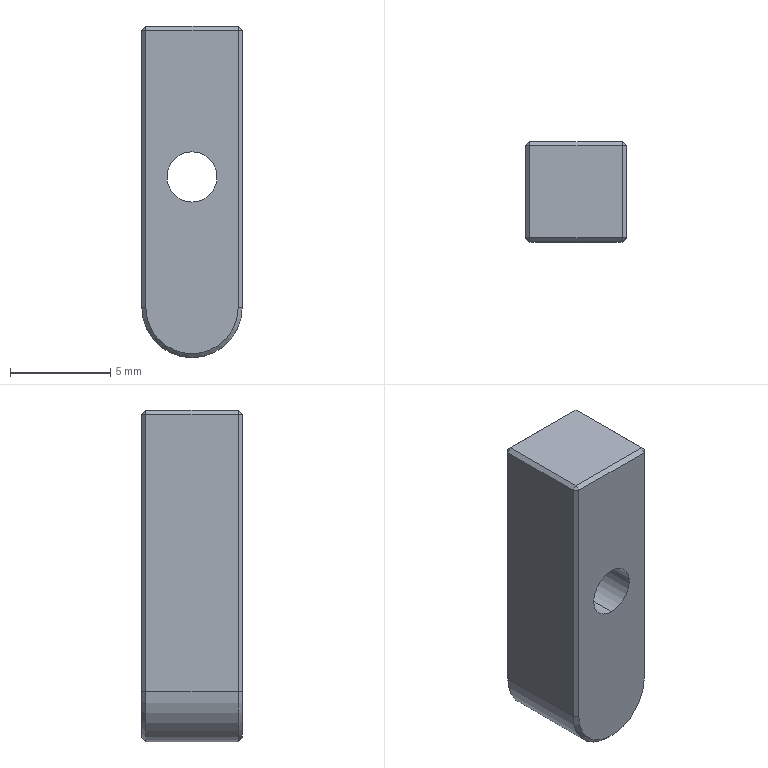Part | STEP file | 22010150--1-SOLI00_1_1_1 | 1 solid | 25 faces | box 5 x 5 x 16.5 mm | volume 372.42 mm3 | plane 17 | cone 5 | cylinder 3 | commonest cylinder face diameters 2.5 x2 5 x1
STEP:
#1=CARTESIAN_POINT('',(0.,0.,0.));
#2=DIRECTION('',(0.,0.,1.));
#3=DIRECTION('',(1.,0.,0.));
#4=AXIS2_PLACEMENT_3D('',#1,#2,#3);
#5=CARTESIAN_POINT('',(0.,4.,23.75));
#6=VERTEX_POINT('',#5);
#7=CARTESIAN_POINT('',(0.,8.725,23.75));
#8=VERTEX_POINT('',#7);
#9=CARTESIAN_POINT('',(0.,9.,23.75));
#10=DIRECTION('',(0.,1.,0.));
#11=VECTOR('',#10,1.);
#12=LINE('',#9,#11);
#13=CARTESIAN_POINT('',(0.,9.,22.5));
#14=DIRECTION('',(0.,1.,0.));
#15=DIRECTION('',(0.,0.,1.));
#16=AXIS2_PLACEMENT_3D('',#13,#14,#15);
#17=CYLINDRICAL_SURFACE('',#16,1.25);
#18=CARTESIAN_POINT('',(6.283,0.));
#19=DIRECTION('',(0.,1.));
#20=VECTOR('',#19,1.);
#21=LINE('',#18,#20);
#22=(GEOMETRIC_REPRESENTATION_CONTEXT(2)PARAMETRIC_REPRESENTATION_CONTEXT()REPRESENTATION_CONTEXT('',''));
#23=DEFINITIONAL_REPRESENTATION('',(#21),#22);
#24=PCURVE('',#17,#23);
#25=CARTESIAN_POINT('',(0.,9.,22.5));
#26=DIRECTION('',(0.,1.,0.));
#27=DIRECTION('',(0.,0.,1.));
#28=AXIS2_PLACEMENT_3D('',#25,#26,#27);
#29=CYLINDRICAL_SURFACE('',#28,1.25);
#30=CARTESIAN_POINT('',(0.,0.));
#31=DIRECTION('',(0.,1.));
#32=VECTOR('',#31,1.);
#33=LINE('',#30,#32);
#34=(GEOMETRIC_REPRESENTATION_CONTEXT(2)PARAMETRIC_REPRESENTATION_CONTEXT()REPRESENTATION_CONTEXT('',''));
#35=DEFINITIONAL_REPRESENTATION('',(#33),#34);
#36=PCURVE('',#29,#35);
#37=SURFACE_CURVE('',#12,(#24,#36),.PCURVE_S1.);
#38=EDGE_CURVE('',#6,#8,#37,.T.);
#39=ORIENTED_EDGE('',*,*,#38,.T.);
#40=CARTESIAN_POINT('',(0.,8.725,21.25));
#41=VERTEX_POINT('',#40);
#42=CARTESIAN_POINT('',(0.,8.725,22.5));
#43=DIRECTION('',(0.,-1.,0.));
#44=DIRECTION('',(0.,0.,1.));
#45=AXIS2_PLACEMENT_3D('',#42,#43,#44);
#46=CIRCLE('',#45,1.25);
#47=CARTESIAN_POINT('',(6.283,-0.275));
#48=DIRECTION('',(-1.,0.));
#49=VECTOR('',#48,1.);
#50=LINE('',#47,#49);
#51=(GEOMETRIC_REPRESENTATION_CONTEXT(2)PARAMETRIC_REPRESENTATION_CONTEXT()REPRESENTATION_CONTEXT('',''));
#52=DEFINITIONAL_REPRESENTATION('',(#50),#51);
#53=PCURVE('',#17,#52);
#54=CARTESIAN_POINT('',(0.,9.,22.5));
#55=DIRECTION('',(0.,1.,0.));
#56=DIRECTION('',(0.,0.,1.));
#57=AXIS2_PLACEMENT_3D('',#54,#55,#56);
#58=CONICAL_SURFACE('',#57,1.525,0.7854);
#59=CARTESIAN_POINT('',(6.283,-0.275));
#60=DIRECTION('',(-1.,0.));
#61=VECTOR('',#60,1.);
#62=LINE('',#59,#61);
#63=(GEOMETRIC_REPRESENTATION_CONTEXT(2)PARAMETRIC_REPRESENTATION_CONTEXT()REPRESENTATION_CONTEXT('',''));
#64=DEFINITIONAL_REPRESENTATION('',(#62),#63);
#65=PCURVE('',#58,#64);
#66=SURFACE_CURVE('',#46,(#53,#65),.PCURVE_S1.);
#67=EDGE_CURVE('',#8,#41,#66,.T.);
#68=ORIENTED_EDGE('',*,*,#67,.T.);
#69=CARTESIAN_POINT('',(0.,4.,21.25));
#70=VERTEX_POINT('',#69);
#71=CARTESIAN_POINT('',(0.,9.,21.25));
#72=DIRECTION('',(0.,1.,0.));
#73=VECTOR('',#72,1.);
#74=LINE('',#71,#73);
#75=CARTESIAN_POINT('',(3.142,0.));
#76=DIRECTION('',(0.,1.));
#77=VECTOR('',#76,1.);
#78=LINE('',#75,#77);
#79=(GEOMETRIC_REPRESENTATION_CONTEXT(2)PARAMETRIC_REPRESENTATION_CONTEXT()REPRESENTATION_CONTEXT('',''));
#80=DEFINITIONAL_REPRESENTATION('',(#78),#79);
#81=PCURVE('',#17,#80);
#82=CARTESIAN_POINT('',(3.142,0.));
#83=DIRECTION('',(0.,1.));
#84=VECTOR('',#83,1.);
#85=LINE('',#82,#84);
#86=(GEOMETRIC_REPRESENTATION_CONTEXT(2)PARAMETRIC_REPRESENTATION_CONTEXT()REPRESENTATION_CONTEXT('',''));
#87=DEFINITIONAL_REPRESENTATION('',(#85),#86);
#88=PCURVE('',#29,#87);
#89=SURFACE_CURVE('',#74,(#81,#88),.PCURVE_S1.);
#90=EDGE_CURVE('',#70,#41,#89,.T.);
#91=ORIENTED_EDGE('',*,*,#90,.F.);
#92=CARTESIAN_POINT('',(0.,4.,22.5));
#93=DIRECTION('',(0.,1.,0.));
#94=DIRECTION('',(0.,0.,1.));
#95=AXIS2_PLACEMENT_3D('',#92,#93,#94);
#96=CIRCLE('',#95,1.25);
#97=CARTESIAN_POINT('',(0.,-5.));
#98=DIRECTION('',(1.,0.));
#99=VECTOR('',#98,1.);
#100=LINE('',#97,#99);
#101=(GEOMETRIC_REPRESENTATION_CONTEXT(2)PARAMETRIC_REPRESENTATION_CONTEXT()REPRESENTATION_CONTEXT('',''));
#102=DEFINITIONAL_REPRESENTATION('',(#100),#101);
#103=PCURVE('',#17,#102);
#104=CARTESIAN_POINT('',(0.,4.,16.));
#105=DIRECTION('',(0.,-1.,0.));
#106=DIRECTION('',(0.,0.,-1.));
#107=AXIS2_PLACEMENT_3D('',#104,#105,#106);
#108=PLANE('',#107);
#109=CARTESIAN_POINT('',(-7.75,0.));
#110=CARTESIAN_POINT('',(-7.75,2.165));
#111=CARTESIAN_POINT('',(-5.875,1.083));
#112=CARTESIAN_POINT('',(-4.,0.));
#113=CARTESIAN_POINT('',(-5.875,-1.083));
#114=CARTESIAN_POINT('',(-7.75,-2.165));
#115=CARTESIAN_POINT('',(-7.75,0.));
#116=(BOUNDED_CURVE()B_SPLINE_CURVE(2,(#109,#110,#111,#112,#113,#114,#115),.UNSPECIFIED.,.T.,.F.)B_SPLINE_CURVE_WITH_KNOTS((1,2,2,2,2,1),(-2.094,0.,2.094,4.189,6.283,8.378),.UNSPECIFIED.)CURVE()GEOMETRIC_REPRESENTATION_ITEM()RATIONAL_B_SPLINE_CURVE((1.,0.5,1.,0.5,1.,0.5,1.))REPRESENTATION_ITEM(''));
#117=(GEOMETRIC_REPRESENTATION_CONTEXT(2)PARAMETRIC_REPRESENTATION_CONTEXT()REPRESENTATION_CONTEXT('',''));
#118=DEFINITIONAL_REPRESENTATION('',(#116),#117);
#119=PCURVE('',#108,#118);
#120=SURFACE_CURVE('',#96,(#103,#119),.PCURVE_S1.);
#121=EDGE_CURVE('',#70,#6,#120,.T.);
#122=ORIENTED_EDGE('',*,*,#121,.T.);
#123=EDGE_LOOP('',(#39,#68,#91,#122));
#124=FACE_BOUND('',#123,.F.);
#125=ADVANCED_FACE('',(#124),#17,.F.);
#126=CARTESIAN_POINT('',(0.,9.,24.025));
#127=VERTEX_POINT('',#126);
#128=CARTESIAN_POINT('',(0.,9.,24.025));
#129=DIRECTION('',(0.,0.7071,0.7071));
#130=VECTOR('',#129,1.);
#131=LINE('',#128,#130);
#132=CARTESIAN_POINT('',(6.283,0.));
#133=DIRECTION('',(0.,1.));
#134=VECTOR('',#133,1.);
#135=LINE('',#132,#134);
#136=(GEOMETRIC_REPRESENTATION_CONTEXT(2)PARAMETRIC_REPRESENTATION_CONTEXT()REPRESENTATION_CONTEXT('',''));
#137=DEFINITIONAL_REPRESENTATION('',(#135),#136);
#138=PCURVE('',#58,#137);
#139=CARTESIAN_POINT('',(0.,9.,22.5));
#140=DIRECTION('',(0.,1.,0.));
#141=DIRECTION('',(0.,0.,1.));
#142=AXIS2_PLACEMENT_3D('',#139,#140,#141);
#143=CONICAL_SURFACE('',#142,1.525,0.7854);
#144=CARTESIAN_POINT('',(0.,0.));
#145=DIRECTION('',(0.,1.));
#146=VECTOR('',#145,1.);
#147=LINE('',#144,#146);
#148=(GEOMETRIC_REPRESENTATION_CONTEXT(2)PARAMETRIC_REPRESENTATION_CONTEXT()REPRESENTATION_CONTEXT('',''));
#149=DEFINITIONAL_REPRESENTATION('',(#147),#148);
#150=PCURVE('',#143,#149);
#151=SURFACE_CURVE('',#131,(#138,#150),.PCURVE_S1.);
#152=EDGE_CURVE('',#8,#127,#151,.T.);
#153=ORIENTED_EDGE('',*,*,#152,.T.);
#154=CARTESIAN_POINT('',(0.,9.,20.975));
#155=VERTEX_POINT('',#154);
#156=CARTESIAN_POINT('',(0.,9.,22.5));
#157=DIRECTION('',(0.,-1.,0.));
#158=DIRECTION('',(0.,0.,1.));
#159=AXIS2_PLACEMENT_3D('',#156,#157,#158);
#160=CIRCLE('',#159,1.525);
#161=CARTESIAN_POINT('',(6.283,0.));
#162=DIRECTION('',(-1.,0.));
#163=VECTOR('',#162,1.);
#164=LINE('',#161,#163);
#165=(GEOMETRIC_REPRESENTATION_CONTEXT(2)PARAMETRIC_REPRESENTATION_CONTEXT()REPRESENTATION_CONTEXT('',''));
#166=DEFINITIONAL_REPRESENTATION('',(#164),#165);
#167=PCURVE('',#58,#166);
#168=CARTESIAN_POINT('',(0.,9.,16.));
#169=DIRECTION('',(0.,-1.,0.));
#170=DIRECTION('',(0.,0.,-1.));
#171=AXIS2_PLACEMENT_3D('',#168,#169,#170);
#172=PLANE('',#171);
#173=CARTESIAN_POINT('',(-6.5,0.));
#174=DIRECTION('',(-1.,0.));
#175=AXIS2_PLACEMENT_2D('',#173,#174);
#176=CIRCLE('',#175,1.525);
#177=(GEOMETRIC_REPRESENTATION_CONTEXT(2)PARAMETRIC_REPRESENTATION_CONTEXT()REPRESENTATION_CONTEXT('',''));
#178=DEFINITIONAL_REPRESENTATION('',(#176),#177);
#179=PCURVE('',#172,#178);
#180=SURFACE_CURVE('',#160,(#167,#179),.PCURVE_S1.);
#181=EDGE_CURVE('',#127,#155,#180,.T.);
#182=ORIENTED_EDGE('',*,*,#181,.T.);
#183=CARTESIAN_POINT('',(0.,9.,20.975));
#184=DIRECTION('',(0.,0.7071,-0.7071));
#185=VECTOR('',#184,1.);
#186=LINE('',#183,#185);
#187=CARTESIAN_POINT('',(3.142,0.));
#188=DIRECTION('',(0.,1.));
#189=VECTOR('',#188,1.);
#190=LINE('',#187,#189);
#191=(GEOMETRIC_REPRESENTATION_CONTEXT(2)PARAMETRIC_REPRESENTATION_CONTEXT()REPRESENTATION_CONTEXT('',''));
#192=DEFINITIONAL_REPRESENTATION('',(#190),#191);
#193=PCURVE('',#58,#192);
#194=CARTESIAN_POINT('',(3.142,0.));
#195=DIRECTION('',(0.,1.));
#196=VECTOR('',#195,1.);
#197=LINE('',#194,#196);
#198=(GEOMETRIC_REPRESENTATION_CONTEXT(2)PARAMETRIC_REPRESENTATION_CONTEXT()REPRESENTATION_CONTEXT('',''));
#199=DEFINITIONAL_REPRESENTATION('',(#197),#198);
#200=PCURVE('',#143,#199);
#201=SURFACE_CURVE('',#186,(#193,#200),.PCURVE_S1.);
#202=EDGE_CURVE('',#41,#155,#201,.T.);
#203=ORIENTED_EDGE('',*,*,#202,.F.);
#204=ORIENTED_EDGE('',*,*,#67,.F.);
#205=EDGE_LOOP('',(#153,#182,#203,#204));
#206=FACE_BOUND('',#205,.F.);
#207=ADVANCED_FACE('',(#206),#58,.F.);
#208=CARTESIAN_POINT('',(-2.3,9.,16.));
#209=VERTEX_POINT('',#208);
#210=CARTESIAN_POINT('',(0.,9.,13.7));
#211=VERTEX_POINT('',#210);
#212=CARTESIAN_POINT('',(0.,9.,16.));
#213=DIRECTION('',(0.,-1.,0.));
#214=DIRECTION('',(0.,0.,-1.));
#215=AXIS2_PLACEMENT_3D('',#212,#213,#214);
#216=CIRCLE('',#215,2.3);
#217=CARTESIAN_POINT('',(0.,8.8,16.));
#218=DIRECTION('',(0.,-1.,0.));
#219=DIRECTION('',(0.,0.,-1.));
#220=AXIS2_PLACEMENT_3D('',#217,#218,#219);
#221=CONICAL_SURFACE('',#220,2.5,0.7854);
#222=CARTESIAN_POINT('',(0.,-0.2));
#223=DIRECTION('',(1.,0.));
#224=VECTOR('',#223,1.);
#225=LINE('',#222,#224);
#226=(GEOMETRIC_REPRESENTATION_CONTEXT(2)PARAMETRIC_REPRESENTATION_CONTEXT()REPRESENTATION_CONTEXT('',''));
#227=DEFINITIONAL_REPRESENTATION('',(#225),#226);
#228=PCURVE('',#221,#227);
#229=CARTESIAN_POINT('',(0.,0.));
#230=DIRECTION('',(1.,0.));
#231=AXIS2_PLACEMENT_2D('',#229,#230);
#232=CIRCLE('',#231,2.3);
#233=(GEOMETRIC_REPRESENTATION_CONTEXT(2)PARAMETRIC_REPRESENTATION_CONTEXT()REPRESENTATION_CONTEXT('',''));
#234=DEFINITIONAL_REPRESENTATION('',(#232),#233);
#235=PCURVE('',#172,#234);
#236=SURFACE_CURVE('',#216,(#228,#235),.PCURVE_S1.);
#237=EDGE_CURVE('',#209,#211,#236,.T.);
#238=ORIENTED_EDGE('',*,*,#237,.T.);
#239=CARTESIAN_POINT('',(0.,8.8,13.5));
#240=VERTEX_POINT('',#239);
#241=CARTESIAN_POINT('',(0.,8.8,13.5));
#242=DIRECTION('',(0.,-0.7071,-0.7071));
#243=VECTOR('',#242,1.);
#244=LINE('',#241,#243);
#245=CARTESIAN_POINT('',(6.283,0.));
#246=DIRECTION('',(0.,1.));
#247=VECTOR('',#246,1.);
#248=LINE('',#245,#247);
#249=(GEOMETRIC_REPRESENTATION_CONTEXT(2)PARAMETRIC_REPRESENTATION_CONTEXT()REPRESENTATION_CONTEXT('',''));
#250=DEFINITIONAL_REPRESENTATION('',(#248),#249);
#251=PCURVE('',#221,#250);
#252=CARTESIAN_POINT('',(0.,8.8,16.));
#253=DIRECTION('',(0.,-1.,0.));
#254=DIRECTION('',(0.,0.,-1.));
#255=AXIS2_PLACEMENT_3D('',#252,#253,#254);
#256=CONICAL_SURFACE('',#255,2.5,0.7854);
#257=CARTESIAN_POINT('',(0.,0.));
#258=DIRECTION('',(0.,1.));
#259=VECTOR('',#258,1.);
#260=LINE('',#257,#259);
#261=(GEOMETRIC_REPRESENTATION_CONTEXT(2)PARAMETRIC_REPRESENTATION_CONTEXT()REPRESENTATION_CONTEXT('',''));
#262=DEFINITIONAL_REPRESENTATION('',(#260),#261);
#263=PCURVE('',#256,#262);
#264=SURFACE_CURVE('',#244,(#251,#263),.PCURVE_S1.);
#265=EDGE_CURVE('',#211,#240,#264,.T.);
#266=ORIENTED_EDGE('',*,*,#265,.T.);
#267=CARTESIAN_POINT('',(-2.5,8.8,16.));
#268=VERTEX_POINT('',#267);
#269=CARTESIAN_POINT('',(0.,8.8,16.));
#270=DIRECTION('',(0.,-1.,0.));
#271=DIRECTION('',(0.,0.,1.));
#272=AXIS2_PLACEMENT_3D('',#269,#270,#271);
#273=CIRCLE('',#272,2.5);
#274=CARTESIAN_POINT('',(3.142,0.));
#275=DIRECTION('',(1.,0.));
#276=VECTOR('',#275,1.);
#277=LINE('',#274,#276);
#278=(GEOMETRIC_REPRESENTATION_CONTEXT(2)PARAMETRIC_REPRESENTATION_CONTEXT()REPRESENTATION_CONTEXT('',''));
#279=DEFINITIONAL_REPRESENTATION('',(#277),#278);
#280=PCURVE('',#221,#279);
#281=CARTESIAN_POINT('',(0.,4.,16.));
#282=DIRECTION('',(0.,1.,0.));
#283=DIRECTION('',(0.,0.,1.));
#284=AXIS2_PLACEMENT_3D('',#281,#282,#283);
#285=CYLINDRICAL_SURFACE('',#284,2.5);
#286=CARTESIAN_POINT('',(6.283,4.8));
#287=DIRECTION('',(-1.,0.));
#288=VECTOR('',#287,1.);
#289=LINE('',#286,#288);
#290=(GEOMETRIC_REPRESENTATION_CONTEXT(2)PARAMETRIC_REPRESENTATION_CONTEXT()REPRESENTATION_CONTEXT('',''));
#291=DEFINITIONAL_REPRESENTATION('',(#289),#290);
#292=PCURVE('',#285,#291);
#293=SURFACE_CURVE('',#273,(#280,#292),.PCURVE_S1.);
#294=EDGE_CURVE('',#268,#240,#293,.T.);
#295=ORIENTED_EDGE('',*,*,#294,.F.);
#296=CARTESIAN_POINT('',(-498984.,-498972.7,16.));
#297=DIRECTION('',(0.7071,0.7071,0.));
#298=VECTOR('',#297,1.);
#299=LINE('',#296,#298);
#300=CARTESIAN_POINT('',(4.712,498981.5));
#301=DIRECTION('',(0.,-1.));
#302=VECTOR('',#301,1.);
#303=LINE('',#300,#302);
#304=(GEOMETRIC_REPRESENTATION_CONTEXT(2)PARAMETRIC_REPRESENTATION_CONTEXT()REPRESENTATION_CONTEXT('',''));
#305=DEFINITIONAL_REPRESENTATION('',(#303),#304);
#306=PCURVE('',#221,#305);
#307=CARTESIAN_POINT('',(-2.5,8.8,16.));
#308=DIRECTION('',(0.7071,-0.7071,0.));
#309=DIRECTION('',(0.7071,0.7071,0.));
#310=AXIS2_PLACEMENT_3D('',#307,#308,#309);
#311=PLANE('',#310);
#312=CARTESIAN_POINT('',(-705666.405,0.));
#313=DIRECTION('',(1.,0.));
#314=VECTOR('',#313,1.);
#315=LINE('',#312,#314);
#316=(GEOMETRIC_REPRESENTATION_CONTEXT(2)PARAMETRIC_REPRESENTATION_CONTEXT()REPRESENTATION_CONTEXT('',''));
#317=DEFINITIONAL_REPRESENTATION('',(#315),#316);
#318=PCURVE('',#311,#317);
#319=SURFACE_CURVE('',#299,(#306,#318),.PCURVE_S1.);
#320=EDGE_CURVE('',#268,#209,#319,.T.);
#321=ORIENTED_EDGE('',*,*,#320,.T.);
#322=EDGE_LOOP('',(#238,#266,#295,#321));
#323=FACE_BOUND('',#322,.T.);
#324=ADVANCED_FACE('',(#323),#221,.T.);
#325=CARTESIAN_POINT('',(0.,4.,22.5));
#326=DIRECTION('',(0.,1.,0.));
#327=DIRECTION('',(0.,0.,1.));
#328=AXIS2_PLACEMENT_3D('',#325,#326,#327);
#329=CIRCLE('',#328,1.25);
#330=CARTESIAN_POINT('',(-7.75,0.));
#331=CARTESIAN_POINT('',(-7.75,2.165));
#332=CARTESIAN_POINT('',(-5.875,1.083));
#333=CARTESIAN_POINT('',(-4.,0.));
#334=CARTESIAN_POINT('',(-5.875,-1.083));
#335=CARTESIAN_POINT('',(-7.75,-2.165));
#336=CARTESIAN_POINT('',(-7.75,0.));
#337=(BOUNDED_CURVE()B_SPLINE_CURVE(2,(#330,#331,#332,#333,#334,#335,#336),.UNSPECIFIED.,.T.,.F.)B_SPLINE_CURVE_WITH_KNOTS((1,2,2,2,2,1),(-2.094,0.,2.094,4.189,6.283,8.378),.UNSPECIFIED.)CURVE()GEOMETRIC_REPRESENTATION_ITEM()RATIONAL_B_SPLINE_CURVE((1.,0.5,1.,0.5,1.,0.5,1.))REPRESENTATION_ITEM(''));
#338=(GEOMETRIC_REPRESENTATION_CONTEXT(2)PARAMETRIC_REPRESENTATION_CONTEXT()REPRESENTATION_CONTEXT('',''));
#339=DEFINITIONAL_REPRESENTATION('',(#337),#338);
#340=PCURVE('',#108,#339);
#341=CARTESIAN_POINT('',(0.,-5.));
#342=DIRECTION('',(1.,0.));
#343=VECTOR('',#342,1.);
#344=LINE('',#341,#343);
#345=(GEOMETRIC_REPRESENTATION_CONTEXT(2)PARAMETRIC_REPRESENTATION_CONTEXT()REPRESENTATION_CONTEXT('',''));
#346=DEFINITIONAL_REPRESENTATION('',(#344),#345);
#347=PCURVE('',#29,#346);
#348=SURFACE_CURVE('',#329,(#340,#347),.PCURVE_S1.);
#349=EDGE_CURVE('',#6,#70,#348,.T.);
#350=ORIENTED_EDGE('',*,*,#349,.T.);
#351=ORIENTED_EDGE('',*,*,#121,.T.);
#352=EDGE_LOOP('',(#350,#351));
#353=FACE_BOUND('',#352,.T.);
#354=CARTESIAN_POINT('',(2.3,4.,16.));
#355=VERTEX_POINT('',#354);
#356=CARTESIAN_POINT('',(2.3,4.,29.8));
#357=VERTEX_POINT('',#356);
#358=CARTESIAN_POINT('',(2.3,4.,16.));
#359=DIRECTION('',(0.,0.,1.));
#360=VECTOR('',#359,1.);
#361=LINE('',#358,#360);
#362=CARTESIAN_POINT('',(0.,2.3));
#363=DIRECTION('',(-1.,0.));
#364=VECTOR('',#363,1.);
#365=LINE('',#362,#364);
#366=(GEOMETRIC_REPRESENTATION_CONTEXT(2)PARAMETRIC_REPRESENTATION_CONTEXT()REPRESENTATION_CONTEXT('',''));
#367=DEFINITIONAL_REPRESENTATION('',(#365),#366);
#368=PCURVE('',#108,#367);
#369=CARTESIAN_POINT('',(2.3,4.,16.));
#370=DIRECTION('',(0.7071,-0.7071,0.));
#371=DIRECTION('',(0.7071,0.7071,0.));
#372=AXIS2_PLACEMENT_3D('',#369,#370,#371);
#373=PLANE('',#372);
#374=CARTESIAN_POINT('',(0.,0.));
#375=DIRECTION('',(0.,1.));
#376=VECTOR('',#375,1.);
#377=LINE('',#374,#376);
#378=(GEOMETRIC_REPRESENTATION_CONTEXT(2)PARAMETRIC_REPRESENTATION_CONTEXT()REPRESENTATION_CONTEXT('',''));
#379=DEFINITIONAL_REPRESENTATION('',(#377),#378);
#380=PCURVE('',#373,#379);
#381=SURFACE_CURVE('',#361,(#368,#380),.PCURVE_S1.);
#382=EDGE_CURVE('',#355,#357,#381,.T.);
#383=ORIENTED_EDGE('',*,*,#382,.T.);
#384=CARTESIAN_POINT('',(-2.3,4.,29.8));
#385=VERTEX_POINT('',#384);
#386=CARTESIAN_POINT('',(0.,4.,29.8));
#387=DIRECTION('',(-1.,0.,0.));
#388=VECTOR('',#387,1.);
#389=LINE('',#386,#388);
#390=CARTESIAN_POINT('',(-13.8,0.));
#391=DIRECTION('',(0.,-1.));
#392=VECTOR('',#391,1.);
#393=LINE('',#390,#392);
#394=(GEOMETRIC_REPRESENTATION_CONTEXT(2)PARAMETRIC_REPRESENTATION_CONTEXT()REPRESENTATION_CONTEXT('',''));
#395=DEFINITIONAL_REPRESENTATION('',(#393),#394);
#396=PCURVE('',#108,#395);
#397=CARTESIAN_POINT('',(0.,4.,29.8));
#398=DIRECTION('',(0.,-0.7071,0.7071));
#399=DIRECTION('',(0.,-0.7071,-0.7071));
#400=AXIS2_PLACEMENT_3D('',#397,#398,#399);
#401=PLANE('',#400);
#402=CARTESIAN_POINT('',(0.,0.));
#403=DIRECTION('',(0.,-1.));
#404=VECTOR('',#403,1.);
#405=LINE('',#402,#404);
#406=(GEOMETRIC_REPRESENTATION_CONTEXT(2)PARAMETRIC_REPRESENTATION_CONTEXT()REPRESENTATION_CONTEXT('',''));
#407=DEFINITIONAL_REPRESENTATION('',(#405),#406);
#408=PCURVE('',#401,#407);
#409=SURFACE_CURVE('',#389,(#396,#408),.PCURVE_S1.);
#410=EDGE_CURVE('',#357,#385,#409,.T.);
#411=ORIENTED_EDGE('',*,*,#410,.T.);
#412=CARTESIAN_POINT('',(-2.3,4.,16.));
#413=VERTEX_POINT('',#412);
#414=CARTESIAN_POINT('',(-2.3,4.,16.));
#415=DIRECTION('',(0.,0.,-1.));
#416=VECTOR('',#415,1.);
#417=LINE('',#414,#416);
#418=CARTESIAN_POINT('',(0.,-2.3));
#419=DIRECTION('',(1.,0.));
#420=VECTOR('',#419,1.);
#421=LINE('',#418,#420);
#422=(GEOMETRIC_REPRESENTATION_CONTEXT(2)PARAMETRIC_REPRESENTATION_CONTEXT()REPRESENTATION_CONTEXT('',''));
#423=DEFINITIONAL_REPRESENTATION('',(#421),#422);
#424=PCURVE('',#108,#423);
#425=CARTESIAN_POINT('',(-2.3,4.,16.));
#426=DIRECTION('',(-0.7071,-0.7071,0.));
#427=DIRECTION('',(0.7071,-0.7071,0.));
#428=AXIS2_PLACEMENT_3D('',#425,#426,#427);
#429=PLANE('',#428);
#430=CARTESIAN_POINT('',(0.,0.));
#431=DIRECTION('',(0.,-1.));
#432=VECTOR('',#431,1.);
#433=LINE('',#430,#432);
#434=(GEOMETRIC_REPRESENTATION_CONTEXT(2)PARAMETRIC_REPRESENTATION_CONTEXT()REPRESENTATION_CONTEXT('',''));
#435=DEFINITIONAL_REPRESENTATION('',(#433),#434);
#436=PCURVE('',#429,#435);
#437=SURFACE_CURVE('',#417,(#424,#436),.PCURVE_S1.);
#438=EDGE_CURVE('',#385,#413,#437,.T.);
#439=ORIENTED_EDGE('',*,*,#438,.T.);
#440=CARTESIAN_POINT('',(0.,4.,16.));
#441=DIRECTION('',(0.,-1.,0.));
#442=DIRECTION('',(0.,0.,1.));
#443=AXIS2_PLACEMENT_3D('',#440,#441,#442);
#444=CIRCLE('',#443,2.3);
#445=CARTESIAN_POINT('',(0.,0.));
#446=DIRECTION('',(-1.,0.));
#447=AXIS2_PLACEMENT_2D('',#445,#446);
#448=CIRCLE('',#447,2.3);
#449=(GEOMETRIC_REPRESENTATION_CONTEXT(2)PARAMETRIC_REPRESENTATION_CONTEXT()REPRESENTATION_CONTEXT('',''));
#450=DEFINITIONAL_REPRESENTATION('',(#448),#449);
#451=PCURVE('',#108,#450);
#452=CARTESIAN_POINT('',(0.,4.2,16.));
#453=DIRECTION('',(0.,1.,0.));
#454=DIRECTION('',(0.,0.,1.));
#455=AXIS2_PLACEMENT_3D('',#452,#453,#454);
#456=CONICAL_SURFACE('',#455,2.5,0.7854);
#457=CARTESIAN_POINT('',(6.283,-0.2));
#458=DIRECTION('',(-1.,0.));
#459=VECTOR('',#458,1.);
#460=LINE('',#457,#459);
#461=(GEOMETRIC_REPRESENTATION_CONTEXT(2)PARAMETRIC_REPRESENTATION_CONTEXT()REPRESENTATION_CONTEXT('',''));
#462=DEFINITIONAL_REPRESENTATION('',(#460),#461);
#463=PCURVE('',#456,#462);
#464=SURFACE_CURVE('',#444,(#451,#463),.PCURVE_S1.);
#465=EDGE_CURVE('',#413,#355,#464,.T.);
#466=ORIENTED_EDGE('',*,*,#465,.T.);
#467=EDGE_LOOP('',(#383,#411,#439,#466));
#468=FACE_BOUND('',#467,.T.);
#469=ADVANCED_FACE('',(#353,#468),#108,.T.);
#470=CARTESIAN_POINT('',(0.,8.725,22.5));
#471=DIRECTION('',(0.,-1.,0.));
#472=DIRECTION('',(0.,0.,1.));
#473=AXIS2_PLACEMENT_3D('',#470,#471,#472);
#474=CIRCLE('',#473,1.25);
#475=CARTESIAN_POINT('',(6.283,-0.275));
#476=DIRECTION('',(-1.,0.));
#477=VECTOR('',#476,1.);
#478=LINE('',#475,#477);
#479=(GEOMETRIC_REPRESENTATION_CONTEXT(2)PARAMETRIC_REPRESENTATION_CONTEXT()REPRESENTATION_CONTEXT('',''));
#480=DEFINITIONAL_REPRESENTATION('',(#478),#479);
#481=PCURVE('',#29,#480);
#482=CARTESIAN_POINT('',(6.283,-0.275));
#483=DIRECTION('',(-1.,0.));
#484=VECTOR('',#483,1.);
#485=LINE('',#482,#484);
#486=(GEOMETRIC_REPRESENTATION_CONTEXT(2)PARAMETRIC_REPRESENTATION_CONTEXT()REPRESENTATION_CONTEXT('',''));
#487=DEFINITIONAL_REPRESENTATION('',(#485),#486);
#488=PCURVE('',#143,#487);
#489=SURFACE_CURVE('',#474,(#481,#488),.PCURVE_S1.);
#490=EDGE_CURVE('',#41,#8,#489,.T.);
#491=ORIENTED_EDGE('',*,*,#490,.T.);
#492=ORIENTED_EDGE('',*,*,#38,.F.);
#493=ORIENTED_EDGE('',*,*,#349,.T.);
#494=ORIENTED_EDGE('',*,*,#90,.T.);
#495=EDGE_LOOP('',(#491,#492,#493,#494));
#496=FACE_BOUND('',#495,.F.);
#497=ADVANCED_FACE('',(#496),#29,.F.);
#498=CARTESIAN_POINT('',(2.3,4.2,30.));
#499=VERTEX_POINT('',#498);
#500=CARTESIAN_POINT('',(-2.3,4.2,30.));
#501=VERTEX_POINT('',#500);
#502=CARTESIAN_POINT('',(0.,4.2,30.));
#503=DIRECTION('',(-1.,0.,0.));
#504=VECTOR('',#503,1.);
#505=LINE('',#502,#504);
#506=CARTESIAN_POINT('',(-0.2828,0.));
#507=DIRECTION('',(0.,-1.));
#508=VECTOR('',#507,1.);
#509=LINE('',#506,#508);
#510=(GEOMETRIC_REPRESENTATION_CONTEXT(2)PARAMETRIC_REPRESENTATION_CONTEXT()REPRESENTATION_CONTEXT('',''));
#511=DEFINITIONAL_REPRESENTATION('',(#509),#510);
#512=PCURVE('',#401,#511);
#513=CARTESIAN_POINT('',(2.5,4.,30.));
#514=DIRECTION('',(0.,0.,-1.));
#515=DIRECTION('',(-1.,0.,0.));
#516=AXIS2_PLACEMENT_3D('',#513,#514,#515);
#517=PLANE('',#516);
#518=CARTESIAN_POINT('',(2.5,0.2));
#519=DIRECTION('',(1.,0.));
#520=VECTOR('',#519,1.);
#521=LINE('',#518,#520);
#522=(GEOMETRIC_REPRESENTATION_CONTEXT(2)PARAMETRIC_REPRESENTATION_CONTEXT()REPRESENTATION_CONTEXT('',''));
#523=DEFINITIONAL_REPRESENTATION('',(#521),#522);
#524=PCURVE('',#517,#523);
#525=SURFACE_CURVE('',#505,(#512,#524),.PCURVE_S1.);
#526=EDGE_CURVE('',#499,#501,#525,.T.);
#527=ORIENTED_EDGE('',*,*,#526,.T.);
#528=CARTESIAN_POINT('',(-2.3,4.,29.8));
#529=DIRECTION('',(0.,-0.7071,-0.7071));
#530=VECTOR('',#529,1.);
#531=LINE('',#528,#530);
#532=CARTESIAN_POINT('',(0.,-2.3));
#533=DIRECTION('',(1.,0.));
#534=VECTOR('',#533,1.);
#535=LINE('',#532,#534);
#536=(GEOMETRIC_REPRESENTATION_CONTEXT(2)PARAMETRIC_REPRESENTATION_CONTEXT()REPRESENTATION_CONTEXT('',''));
#537=DEFINITIONAL_REPRESENTATION('',(#535),#536);
#538=PCURVE('',#401,#537);
#539=CARTESIAN_POINT('',(-2.3,4.2,30.));
#540=DIRECTION('',(-0.5774,-0.5774,0.5774));
#541=DIRECTION('',(0.7071,0.,0.7071));
#542=AXIS2_PLACEMENT_3D('',#539,#540,#541);
#543=PLANE('',#542);
#544=CARTESIAN_POINT('',(-0.1414,-0.2449));
#545=DIRECTION('',(-0.5,-0.866));
#546=VECTOR('',#545,1.);
#547=LINE('',#544,#546);
#548=(GEOMETRIC_REPRESENTATION_CONTEXT(2)PARAMETRIC_REPRESENTATION_CONTEXT()REPRESENTATION_CONTEXT('',''));
#549=DEFINITIONAL_REPRESENTATION('',(#547),#548);
#550=PCURVE('',#543,#549);
#551=SURFACE_CURVE('',#531,(#538,#550),.PCURVE_S1.);
#552=EDGE_CURVE('',#501,#385,#551,.T.);
#553=ORIENTED_EDGE('',*,*,#552,.T.);
#554=ORIENTED_EDGE('',*,*,#410,.F.);
#555=CARTESIAN_POINT('',(2.3,4.,29.8));
#556=DIRECTION('',(0.,0.7071,0.7071));
#557=VECTOR('',#556,1.);
#558=LINE('',#555,#557);
#559=CARTESIAN_POINT('',(0.,2.3));
#560=DIRECTION('',(-1.,0.));
#561=VECTOR('',#560,1.);
#562=LINE('',#559,#561);
#563=(GEOMETRIC_REPRESENTATION_CONTEXT(2)PARAMETRIC_REPRESENTATION_CONTEXT()REPRESENTATION_CONTEXT('',''));
#564=DEFINITIONAL_REPRESENTATION('',(#562),#563);
#565=PCURVE('',#401,#564);
#566=CARTESIAN_POINT('',(2.5,4.2,29.8));
#567=DIRECTION('',(0.5774,-0.5774,0.5774));
#568=DIRECTION('',(0.,-0.7071,-0.7071));
#569=AXIS2_PLACEMENT_3D('',#566,#567,#568);
#570=PLANE('',#569);
#571=CARTESIAN_POINT('',(0.1414,-0.2449));
#572=DIRECTION('',(-1.,0.));
#573=VECTOR('',#572,1.);
#574=LINE('',#571,#573);
#575=(GEOMETRIC_REPRESENTATION_CONTEXT(2)PARAMETRIC_REPRESENTATION_CONTEXT()REPRESENTATION_CONTEXT('',''));
#576=DEFINITIONAL_REPRESENTATION('',(#574),#575);
#577=PCURVE('',#570,#576);
#578=SURFACE_CURVE('',#558,(#565,#577),.PCURVE_S1.);
#579=EDGE_CURVE('',#357,#499,#578,.T.);
#580=ORIENTED_EDGE('',*,*,#579,.T.);
#581=EDGE_LOOP('',(#527,#553,#554,#580));
#582=FACE_BOUND('',#581,.T.);
#583=ADVANCED_FACE('',(#582),#401,.T.);
#584=ORIENTED_EDGE('',*,*,#382,.F.);
#585=CARTESIAN_POINT('',(2.5,4.2,16.));
#586=VERTEX_POINT('',#585);
#587=CARTESIAN_POINT('',(2.3,4.,16.));
#588=DIRECTION('',(0.7071,0.7071,0.));
#589=VECTOR('',#588,1.);
#590=LINE('',#587,#589);
#591=CARTESIAN_POINT('',(0.,0.));
#592=DIRECTION('',(1.,0.));
#593=VECTOR('',#592,1.);
#594=LINE('',#591,#593);
#595=(GEOMETRIC_REPRESENTATION_CONTEXT(2)PARAMETRIC_REPRESENTATION_CONTEXT()REPRESENTATION_CONTEXT('',''));
#596=DEFINITIONAL_REPRESENTATION('',(#594),#595);
#597=PCURVE('',#373,#596);
#598=CARTESIAN_POINT('',(1.571,-0.2));
#599=DIRECTION('',(0.,1.));
#600=VECTOR('',#599,1.);
#601=LINE('',#598,#600);
#602=(GEOMETRIC_REPRESENTATION_CONTEXT(2)PARAMETRIC_REPRESENTATION_CONTEXT()REPRESENTATION_CONTEXT('',''));
#603=DEFINITIONAL_REPRESENTATION('',(#601),#602);
#604=PCURVE('',#456,#603);
#605=SURFACE_CURVE('',#590,(#597,#604),.PCURVE_S1.);
#606=EDGE_CURVE('',#355,#586,#605,.T.);
#607=ORIENTED_EDGE('',*,*,#606,.T.);
#608=CARTESIAN_POINT('',(2.5,4.2,29.8));
#609=VERTEX_POINT('',#608);
#610=CARTESIAN_POINT('',(2.5,4.2,16.));
#611=DIRECTION('',(0.,0.,1.));
#612=VECTOR('',#611,1.);
#613=LINE('',#610,#612);
#614=CARTESIAN_POINT('',(0.2828,0.));
#615=DIRECTION('',(0.,1.));
#616=VECTOR('',#615,1.);
#617=LINE('',#614,#616);
#618=(GEOMETRIC_REPRESENTATION_CONTEXT(2)PARAMETRIC_REPRESENTATION_CONTEXT()REPRESENTATION_CONTEXT('',''));
#619=DEFINITIONAL_REPRESENTATION('',(#617),#618);
#620=PCURVE('',#373,#619);
#621=CARTESIAN_POINT('',(2.5,4.,16.));
#622=DIRECTION('',(-1.,0.,0.));
#623=DIRECTION('',(0.,0.,1.));
#624=AXIS2_PLACEMENT_3D('',#621,#622,#623);
#625=PLANE('',#624);
#626=CARTESIAN_POINT('',(0.,0.2));
#627=DIRECTION('',(1.,0.));
#628=VECTOR('',#627,1.);
#629=LINE('',#626,#628);
#630=(GEOMETRIC_REPRESENTATION_CONTEXT(2)PARAMETRIC_REPRESENTATION_CONTEXT()REPRESENTATION_CONTEXT('',''));
#631=DEFINITIONAL_REPRESENTATION('',(#629),#630);
#632=PCURVE('',#625,#631);
#633=SURFACE_CURVE('',#613,(#620,#632),.PCURVE_S1.);
#634=EDGE_CURVE('',#586,#609,#633,.T.);
#635=ORIENTED_EDGE('',*,*,#634,.T.);
#636=CARTESIAN_POINT('',(2.3,4.,29.8));
#637=DIRECTION('',(-0.7071,-0.7071,0.));
#638=VECTOR('',#637,1.);
#639=LINE('',#636,#638);
#640=CARTESIAN_POINT('',(0.,13.8));
#641=DIRECTION('',(-1.,0.));
#642=VECTOR('',#641,1.);
#643=LINE('',#640,#642);
#644=(GEOMETRIC_REPRESENTATION_CONTEXT(2)PARAMETRIC_REPRESENTATION_CONTEXT()REPRESENTATION_CONTEXT('',''));
#645=DEFINITIONAL_REPRESENTATION('',(#643),#644);
#646=PCURVE('',#373,#645);
#647=CARTESIAN_POINT('',(0.1414,-0.2449));
#648=DIRECTION('',(0.5,-0.866));
#649=VECTOR('',#648,1.);
#650=LINE('',#647,#649);
#651=(GEOMETRIC_REPRESENTATION_CONTEXT(2)PARAMETRIC_REPRESENTATION_CONTEXT()REPRESENTATION_CONTEXT('',''));
#652=DEFINITIONAL_REPRESENTATION('',(#650),#651);
#653=PCURVE('',#570,#652);
#654=SURFACE_CURVE('',#639,(#646,#653),.PCURVE_S1.);
#655=EDGE_CURVE('',#609,#357,#654,.T.);
#656=ORIENTED_EDGE('',*,*,#655,.T.);
#657=EDGE_LOOP('',(#584,#607,#635,#656));
#658=FACE_BOUND('',#657,.T.);
#659=ADVANCED_FACE('',(#658),#373,.T.);
#660=ORIENTED_EDGE('',*,*,#606,.F.);
#661=ORIENTED_EDGE('',*,*,#465,.F.);
#662=CARTESIAN_POINT('',(-2.5,4.2,16.));
#663=VERTEX_POINT('',#662);
#664=CARTESIAN_POINT('',(-498998.3,499000.,16.));
#665=DIRECTION('',(-0.7071,0.7071,0.));
#666=VECTOR('',#665,1.);
#667=LINE('',#664,#666);
#668=CARTESIAN_POINT('',(4.712,498995.8));
#669=DIRECTION('',(0.,1.));
#670=VECTOR('',#669,1.);
#671=LINE('',#668,#670);
#672=(GEOMETRIC_REPRESENTATION_CONTEXT(2)PARAMETRIC_REPRESENTATION_CONTEXT()REPRESENTATION_CONTEXT('',''));
#673=DEFINITIONAL_REPRESENTATION('',(#671),#672);
#674=PCURVE('',#456,#673);
#675=CARTESIAN_POINT('',(-705686.911,-0.000000552));
#676=DIRECTION('',(-1.,0.));
#677=VECTOR('',#676,1.);
#678=LINE('',#675,#677);
#679=(GEOMETRIC_REPRESENTATION_CONTEXT(2)PARAMETRIC_REPRESENTATION_CONTEXT()REPRESENTATION_CONTEXT('',''));
#680=DEFINITIONAL_REPRESENTATION('',(#678),#679);
#681=PCURVE('',#429,#680);
#682=SURFACE_CURVE('',#667,(#674,#681),.PCURVE_S1.);
#683=EDGE_CURVE('',#413,#663,#682,.T.);
#684=ORIENTED_EDGE('',*,*,#683,.T.);
#685=CARTESIAN_POINT('',(0.,4.2,16.));
#686=DIRECTION('',(0.,-1.,0.));
#687=DIRECTION('',(0.,0.,-1.));
#688=AXIS2_PLACEMENT_3D('',#685,#686,#687);
#689=CIRCLE('',#688,2.5);
#690=CARTESIAN_POINT('',(9.425,0.));
#691=DIRECTION('',(-1.,0.));
#692=VECTOR('',#691,1.);
#693=LINE('',#690,#692);
#694=(GEOMETRIC_REPRESENTATION_CONTEXT(2)PARAMETRIC_REPRESENTATION_CONTEXT()REPRESENTATION_CONTEXT('',''));
#695=DEFINITIONAL_REPRESENTATION('',(#693),#694);
#696=PCURVE('',#456,#695);
#697=CARTESIAN_POINT('',(9.425,0.2));
#698=DIRECTION('',(-1.,0.));
#699=VECTOR('',#698,1.);
#700=LINE('',#697,#699);
#701=(GEOMETRIC_REPRESENTATION_CONTEXT(2)PARAMETRIC_REPRESENTATION_CONTEXT()REPRESENTATION_CONTEXT('',''));
#702=DEFINITIONAL_REPRESENTATION('',(#700),#701);
#703=PCURVE('',#285,#702);
#704=SURFACE_CURVE('',#689,(#696,#703),.PCURVE_S1.);
#705=EDGE_CURVE('',#663,#586,#704,.T.);
#706=ORIENTED_EDGE('',*,*,#705,.T.);
#707=EDGE_LOOP('',(#660,#661,#684,#706));
#708=FACE_BOUND('',#707,.T.);
#709=ADVANCED_FACE('',(#708),#456,.T.);
#710=ORIENTED_EDGE('',*,*,#438,.F.);
#711=CARTESIAN_POINT('',(-2.5,4.2,29.8));
#712=VERTEX_POINT('',#711);
#713=CARTESIAN_POINT('',(-2.3,4.,29.8));
#714=DIRECTION('',(-0.7071,0.7071,0.));
#715=VECTOR('',#714,1.);
#716=LINE('',#713,#715);
#717=CARTESIAN_POINT('',(0.,13.8));
#718=DIRECTION('',(-1.,0.));
#719=VECTOR('',#718,1.);
#720=LINE('',#717,#719);
#721=(GEOMETRIC_REPRESENTATION_CONTEXT(2)PARAMETRIC_REPRESENTATION_CONTEXT()REPRESENTATION_CONTEXT('',''));
#722=DEFINITIONAL_REPRESENTATION('',(#720),#721);
#723=PCURVE('',#429,#722);
#724=CARTESIAN_POINT('',(-0.1414,-0.2449));
#725=DIRECTION('',(-0.5,0.866));
#726=VECTOR('',#725,1.);
#727=LINE('',#724,#726);
#728=(GEOMETRIC_REPRESENTATION_CONTEXT(2)PARAMETRIC_REPRESENTATION_CONTEXT()REPRESENTATION_CONTEXT('',''));
#729=DEFINITIONAL_REPRESENTATION('',(#727),#728);
#730=PCURVE('',#543,#729);
#731=SURFACE_CURVE('',#716,(#723,#730),.PCURVE_S1.);
#732=EDGE_CURVE('',#385,#712,#731,.T.);
#733=ORIENTED_EDGE('',*,*,#732,.T.);
#734=CARTESIAN_POINT('',(-2.5,4.2,16.));
#735=DIRECTION('',(0.,0.,-1.));
#736=VECTOR('',#735,1.);
#737=LINE('',#734,#736);
#738=CARTESIAN_POINT('',(-0.2828,0.));
#739=DIRECTION('',(0.,-1.));
#740=VECTOR('',#739,1.);
#741=LINE('',#738,#740);
#742=(GEOMETRIC_REPRESENTATION_CONTEXT(2)PARAMETRIC_REPRESENTATION_CONTEXT()REPRESENTATION_CONTEXT('',''));
#743=DEFINITIONAL_REPRESENTATION('',(#741),#742);
#744=PCURVE('',#429,#743);
#745=CARTESIAN_POINT('',(-2.5,4.,16.));
#746=DIRECTION('',(1.,0.,0.));
#747=DIRECTION('',(0.,0.,-1.));
#748=AXIS2_PLACEMENT_3D('',#745,#746,#747);
#749=PLANE('',#748);
#750=CARTESIAN_POINT('',(0.,0.2));
#751=DIRECTION('',(1.,0.));
#752=VECTOR('',#751,1.);
#753=LINE('',#750,#752);
#754=(GEOMETRIC_REPRESENTATION_CONTEXT(2)PARAMETRIC_REPRESENTATION_CONTEXT()REPRESENTATION_CONTEXT('',''));
#755=DEFINITIONAL_REPRESENTATION('',(#753),#754);
#756=PCURVE('',#749,#755);
#757=SURFACE_CURVE('',#737,(#744,#756),.PCURVE_S1.);
#758=EDGE_CURVE('',#712,#663,#757,.T.);
#759=ORIENTED_EDGE('',*,*,#758,.T.);
#760=ORIENTED_EDGE('',*,*,#683,.F.);
#761=EDGE_LOOP('',(#710,#733,#759,#760));
#762=FACE_BOUND('',#761,.T.);
#763=ADVANCED_FACE('',(#762),#429,.T.);
#764=CARTESIAN_POINT('',(0.,9.,22.5));
#765=DIRECTION('',(0.,-1.,0.));
#766=DIRECTION('',(0.,0.,1.));
#767=AXIS2_PLACEMENT_3D('',#764,#765,#766);
#768=CIRCLE('',#767,1.525);
#769=CARTESIAN_POINT('',(6.283,0.));
#770=DIRECTION('',(-1.,0.));
#771=VECTOR('',#770,1.);
#772=LINE('',#769,#771);
#773=(GEOMETRIC_REPRESENTATION_CONTEXT(2)PARAMETRIC_REPRESENTATION_CONTEXT()REPRESENTATION_CONTEXT('',''));
#774=DEFINITIONAL_REPRESENTATION('',(#772),#773);
#775=PCURVE('',#143,#774);
#776=CARTESIAN_POINT('',(-6.5,0.));
#777=DIRECTION('',(-1.,0.));
#778=AXIS2_PLACEMENT_2D('',#776,#777);
#779=CIRCLE('',#778,1.525);
#780=(GEOMETRIC_REPRESENTATION_CONTEXT(2)PARAMETRIC_REPRESENTATION_CONTEXT()REPRESENTATION_CONTEXT('',''));
#781=DEFINITIONAL_REPRESENTATION('',(#779),#780);
#782=PCURVE('',#172,#781);
#783=SURFACE_CURVE('',#768,(#775,#782),.PCURVE_S1.);
#784=EDGE_CURVE('',#155,#127,#783,.T.);
#785=ORIENTED_EDGE('',*,*,#784,.T.);
#786=ORIENTED_EDGE('',*,*,#152,.F.);
#787=ORIENTED_EDGE('',*,*,#490,.F.);
#788=ORIENTED_EDGE('',*,*,#202,.T.);
#789=EDGE_LOOP('',(#785,#786,#787,#788));
#790=FACE_BOUND('',#789,.F.);
#791=ADVANCED_FACE('',(#790),#143,.F.);
#792=ORIENTED_EDGE('',*,*,#552,.F.);
#793=CARTESIAN_POINT('',(-2.5,4.2,29.8));
#794=DIRECTION('',(-0.7071,0.,-0.7071));
#795=VECTOR('',#794,1.);
#796=LINE('',#793,#795);
#797=CARTESIAN_POINT('',(-0.2828,0.));
#798=DIRECTION('',(-1.,0.));
#799=VECTOR('',#798,1.);
#800=LINE('',#797,#799);
#801=(GEOMETRIC_REPRESENTATION_CONTEXT(2)PARAMETRIC_REPRESENTATION_CONTEXT()REPRESENTATION_CONTEXT('',''));
#802=DEFINITIONAL_REPRESENTATION('',(#800),#801);
#803=PCURVE('',#543,#802);
#804=CARTESIAN_POINT('',(-2.5,4.,29.8));
#805=DIRECTION('',(0.7071,0.,-0.7071));
#806=DIRECTION('',(-0.7071,0.,-0.7071));
#807=AXIS2_PLACEMENT_3D('',#804,#805,#806);
#808=PLANE('',#807);
#809=CARTESIAN_POINT('',(0.,0.2));
#810=DIRECTION('',(1.,0.));
#811=VECTOR('',#810,1.);
#812=LINE('',#809,#811);
#813=(GEOMETRIC_REPRESENTATION_CONTEXT(2)PARAMETRIC_REPRESENTATION_CONTEXT()REPRESENTATION_CONTEXT('',''));
#814=DEFINITIONAL_REPRESENTATION('',(#812),#813);
#815=PCURVE('',#808,#814);
#816=SURFACE_CURVE('',#796,(#803,#815),.PCURVE_S1.);
#817=EDGE_CURVE('',#501,#712,#816,.T.);
#818=ORIENTED_EDGE('',*,*,#817,.T.);
#819=ORIENTED_EDGE('',*,*,#732,.F.);
#820=EDGE_LOOP('',(#792,#818,#819));
#821=FACE_BOUND('',#820,.T.);
#822=ADVANCED_FACE('',(#821),#543,.T.);
#823=CARTESIAN_POINT('',(-2.3,8.8,30.));
#824=VERTEX_POINT('',#823);
#825=CARTESIAN_POINT('',(2.3,8.8,30.));
#826=VERTEX_POINT('',#825);
#827=CARTESIAN_POINT('',(2.5,8.8,30.));
#828=DIRECTION('',(1.,0.,0.));
#829=VECTOR('',#828,1.);
#830=LINE('',#827,#829);
#831=CARTESIAN_POINT('',(0.,4.8));
#832=DIRECTION('',(-1.,0.));
#833=VECTOR('',#832,1.);
#834=LINE('',#831,#833);
#835=(GEOMETRIC_REPRESENTATION_CONTEXT(2)PARAMETRIC_REPRESENTATION_CONTEXT()REPRESENTATION_CONTEXT('',''));
#836=DEFINITIONAL_REPRESENTATION('',(#834),#835);
#837=PCURVE('',#517,#836);
#838=CARTESIAN_POINT('',(2.5,8.8,30.));
#839=DIRECTION('',(0.,-0.7071,-0.7071));
#840=DIRECTION('',(0.,0.7071,-0.7071));
#841=AXIS2_PLACEMENT_3D('',#838,#839,#840);
#842=PLANE('',#841);
#843=CARTESIAN_POINT('',(0.,0.));
#844=DIRECTION('',(0.,1.));
#845=VECTOR('',#844,1.);
#846=LINE('',#843,#845);
#847=(GEOMETRIC_REPRESENTATION_CONTEXT(2)PARAMETRIC_REPRESENTATION_CONTEXT()REPRESENTATION_CONTEXT('',''));
#848=DEFINITIONAL_REPRESENTATION('',(#846),#847);
#849=PCURVE('',#842,#848);
#850=SURFACE_CURVE('',#830,(#837,#849),.PCURVE_S1.);
#851=EDGE_CURVE('',#824,#826,#850,.T.);
#852=ORIENTED_EDGE('',*,*,#851,.F.);
#853=CARTESIAN_POINT('',(-2.3,4.,30.));
#854=DIRECTION('',(0.,1.,0.));
#855=VECTOR('',#854,1.);
#856=LINE('',#853,#855);
#857=CARTESIAN_POINT('',(4.8,0.));
#858=DIRECTION('',(0.,1.));
#859=VECTOR('',#858,1.);
#860=LINE('',#857,#859);
#861=(GEOMETRIC_REPRESENTATION_CONTEXT(2)PARAMETRIC_REPRESENTATION_CONTEXT()REPRESENTATION_CONTEXT('',''));
#862=DEFINITIONAL_REPRESENTATION('',(#860),#861);
#863=PCURVE('',#517,#862);
#864=CARTESIAN_POINT('',(-0.2828,0.));
#865=DIRECTION('',(0.,1.));
#866=VECTOR('',#865,1.);
#867=LINE('',#864,#866);
#868=(GEOMETRIC_REPRESENTATION_CONTEXT(2)PARAMETRIC_REPRESENTATION_CONTEXT()REPRESENTATION_CONTEXT('',''));
#869=DEFINITIONAL_REPRESENTATION('',(#867),#868);
#870=PCURVE('',#808,#869);
#871=SURFACE_CURVE('',#856,(#863,#870),.PCURVE_S1.);
#872=EDGE_CURVE('',#501,#824,#871,.T.);
#873=ORIENTED_EDGE('',*,*,#872,.F.);
#874=ORIENTED_EDGE('',*,*,#526,.F.);
#875=CARTESIAN_POINT('',(2.3,4.,30.));
#876=DIRECTION('',(0.,-1.,0.));
#877=VECTOR('',#876,1.);
#878=LINE('',#875,#877);
#879=CARTESIAN_POINT('',(0.2,0.));
#880=DIRECTION('',(0.,-1.));
#881=VECTOR('',#880,1.);
#882=LINE('',#879,#881);
#883=(GEOMETRIC_REPRESENTATION_CONTEXT(2)PARAMETRIC_REPRESENTATION_CONTEXT()REPRESENTATION_CONTEXT('',''));
#884=DEFINITIONAL_REPRESENTATION('',(#882),#883);
#885=PCURVE('',#517,#884);
#886=CARTESIAN_POINT('',(2.3,4.,30.));
#887=DIRECTION('',(-0.7071,0.,-0.7071));
#888=DIRECTION('',(-0.7071,0.,0.7071));
#889=AXIS2_PLACEMENT_3D('',#886,#887,#888);
#890=PLANE('',#889);
#891=CARTESIAN_POINT('',(0.,0.));
#892=DIRECTION('',(0.,-1.));
#893=VECTOR('',#892,1.);
#894=LINE('',#891,#893);
#895=(GEOMETRIC_REPRESENTATION_CONTEXT(2)PARAMETRIC_REPRESENTATION_CONTEXT()REPRESENTATION_CONTEXT('',''));
#896=DEFINITIONAL_REPRESENTATION('',(#894),#895);
#897=PCURVE('',#890,#896);
#898=SURFACE_CURVE('',#878,(#885,#897),.PCURVE_S1.);
#899=EDGE_CURVE('',#826,#499,#898,.T.);
#900=ORIENTED_EDGE('',*,*,#899,.F.);
#901=EDGE_LOOP('',(#852,#873,#874,#900));
#902=FACE_BOUND('',#901,.T.);
#903=ADVANCED_FACE('',(#902),#517,.F.);
#904=CARTESIAN_POINT('',(2.5,4.2,29.8));
#905=DIRECTION('',(-0.7071,0.,0.7071));
#906=VECTOR('',#905,1.);
#907=LINE('',#904,#906);
#908=CARTESIAN_POINT('',(0.,0.));
#909=DIRECTION('',(-0.5,-0.866));
#910=VECTOR('',#909,1.);
#911=LINE('',#908,#910);
#912=(GEOMETRIC_REPRESENTATION_CONTEXT(2)PARAMETRIC_REPRESENTATION_CONTEXT()REPRESENTATION_CONTEXT('',''));
#913=DEFINITIONAL_REPRESENTATION('',(#911),#912);
#914=PCURVE('',#570,#913);
#915=CARTESIAN_POINT('',(-0.2828,0.2));
#916=DIRECTION('',(1.,0.));
#917=VECTOR('',#916,1.);
#918=LINE('',#915,#917);
#919=(GEOMETRIC_REPRESENTATION_CONTEXT(2)PARAMETRIC_REPRESENTATION_CONTEXT()REPRESENTATION_CONTEXT('',''));
#920=DEFINITIONAL_REPRESENTATION('',(#918),#919);
#921=PCURVE('',#890,#920);
#922=SURFACE_CURVE('',#907,(#914,#921),.PCURVE_S1.);
#923=EDGE_CURVE('',#609,#499,#922,.T.);
#924=ORIENTED_EDGE('',*,*,#923,.T.);
#925=ORIENTED_EDGE('',*,*,#579,.F.);
#926=ORIENTED_EDGE('',*,*,#655,.F.);
#927=EDGE_LOOP('',(#924,#925,#926));
#928=FACE_BOUND('',#927,.T.);
#929=ADVANCED_FACE('',(#928),#570,.T.);
#930=CARTESIAN_POINT('',(2.5,8.8,29.8));
#931=VERTEX_POINT('',#930);
#932=CARTESIAN_POINT('',(2.5,4.,29.8));
#933=DIRECTION('',(0.,1.,0.));
#934=VECTOR('',#933,1.);
#935=LINE('',#932,#934);
#936=CARTESIAN_POINT('',(13.8,0.));
#937=DIRECTION('',(0.,1.));
#938=VECTOR('',#937,1.);
#939=LINE('',#936,#938);
#940=(GEOMETRIC_REPRESENTATION_CONTEXT(2)PARAMETRIC_REPRESENTATION_CONTEXT()REPRESENTATION_CONTEXT('',''));
#941=DEFINITIONAL_REPRESENTATION('',(#939),#940);
#942=PCURVE('',#625,#941);
#943=CARTESIAN_POINT('',(-0.2828,0.));
#944=DIRECTION('',(0.,1.));
#945=VECTOR('',#944,1.);
#946=LINE('',#943,#945);
#947=(GEOMETRIC_REPRESENTATION_CONTEXT(2)PARAMETRIC_REPRESENTATION_CONTEXT()REPRESENTATION_CONTEXT('',''));
#948=DEFINITIONAL_REPRESENTATION('',(#946),#947);
#949=PCURVE('',#890,#948);
#950=SURFACE_CURVE('',#935,(#942,#949),.PCURVE_S1.);
#951=EDGE_CURVE('',#609,#931,#950,.T.);
#952=ORIENTED_EDGE('',*,*,#951,.F.);
#953=ORIENTED_EDGE('',*,*,#634,.F.);
#954=CARTESIAN_POINT('',(2.5,8.8,16.));
#955=VERTEX_POINT('',#954);
#956=CARTESIAN_POINT('',(2.5,4.,16.));
#957=DIRECTION('',(0.,-1.,0.));
#958=VECTOR('',#957,1.);
#959=LINE('',#956,#958);
#960=CARTESIAN_POINT('',(0.,0.));
#961=DIRECTION('',(0.,-1.));
#962=VECTOR('',#961,1.);
#963=LINE('',#960,#962);
#964=(GEOMETRIC_REPRESENTATION_CONTEXT(2)PARAMETRIC_REPRESENTATION_CONTEXT()REPRESENTATION_CONTEXT('',''));
#965=DEFINITIONAL_REPRESENTATION('',(#963),#964);
#966=PCURVE('',#625,#965);
#967=CARTESIAN_POINT('',(1.571,0.));
#968=DIRECTION('',(0.,-1.));
#969=VECTOR('',#968,1.);
#970=LINE('',#967,#969);
#971=(GEOMETRIC_REPRESENTATION_CONTEXT(2)PARAMETRIC_REPRESENTATION_CONTEXT()REPRESENTATION_CONTEXT('',''));
#972=DEFINITIONAL_REPRESENTATION('',(#970),#971);
#973=PCURVE('',#285,#972);
#974=SURFACE_CURVE('',#959,(#966,#973),.PCURVE_S1.);
#975=EDGE_CURVE('',#955,#586,#974,.T.);
#976=ORIENTED_EDGE('',*,*,#975,.F.);
#977=CARTESIAN_POINT('',(2.5,8.8,16.));
#978=DIRECTION('',(0.,0.,-1.));
#979=VECTOR('',#978,1.);
#980=LINE('',#977,#979);
#981=CARTESIAN_POINT('',(0.,4.8));
#982=DIRECTION('',(-1.,0.));
#983=VECTOR('',#982,1.);
#984=LINE('',#981,#983);
#985=(GEOMETRIC_REPRESENTATION_CONTEXT(2)PARAMETRIC_REPRESENTATION_CONTEXT()REPRESENTATION_CONTEXT('',''));
#986=DEFINITIONAL_REPRESENTATION('',(#984),#985);
#987=PCURVE('',#625,#986);
#988=CARTESIAN_POINT('',(2.5,8.8,16.));
#989=DIRECTION('',(-0.7071,-0.7071,0.));
#990=DIRECTION('',(0.7071,-0.7071,0.));
#991=AXIS2_PLACEMENT_3D('',#988,#989,#990);
#992=PLANE('',#991);
#993=CARTESIAN_POINT('',(0.,0.));
#994=DIRECTION('',(0.,-1.));
#995=VECTOR('',#994,1.);
#996=LINE('',#993,#995);
#997=(GEOMETRIC_REPRESENTATION_CONTEXT(2)PARAMETRIC_REPRESENTATION_CONTEXT()REPRESENTATION_CONTEXT('',''));
#998=DEFINITIONAL_REPRESENTATION('',(#996),#997);
#999=PCURVE('',#992,#998);
#1000=SURFACE_CURVE('',#980,(#987,#999),.PCURVE_S1.);
#1001=EDGE_CURVE('',#931,#955,#1000,.T.);
#1002=ORIENTED_EDGE('',*,*,#1001,.F.);
#1003=EDGE_LOOP('',(#952,#953,#976,#1002));
#1004=FACE_BOUND('',#1003,.T.);
#1005=ADVANCED_FACE('',(#1004),#625,.F.);
#1006=ORIENTED_EDGE('',*,*,#975,.T.);
#1007=ORIENTED_EDGE('',*,*,#705,.F.);
#1008=CARTESIAN_POINT('',(-2.5,4.,16.));
#1009=DIRECTION('',(0.,1.,0.));
#1010=VECTOR('',#1009,1.);
#1011=LINE('',#1008,#1010);
#1012=CARTESIAN_POINT('',(4.712,0.));
#1013=DIRECTION('',(0.,1.));
#1014=VECTOR('',#1013,1.);
#1015=LINE('',#1012,#1014);
#1016=(GEOMETRIC_REPRESENTATION_CONTEXT(2)PARAMETRIC_REPRESENTATION_CONTEXT()REPRESENTATION_CONTEXT('',''));
#1017=DEFINITIONAL_REPRESENTATION('',(#1015),#1016);
#1018=PCURVE('',#285,#1017);
#1019=CARTESIAN_POINT('',(0.,0.));
#1020=DIRECTION('',(0.,1.));
#1021=VECTOR('',#1020,1.);
#1022=LINE('',#1019,#1021);
#1023=(GEOMETRIC_REPRESENTATION_CONTEXT(2)PARAMETRIC_REPRESENTATION_CONTEXT()REPRESENTATION_CONTEXT('',''));
#1024=DEFINITIONAL_REPRESENTATION('',(#1022),#1023);
#1025=PCURVE('',#749,#1024);
#1026=SURFACE_CURVE('',#1011,(#1018,#1025),.PCURVE_S1.);
#1027=EDGE_CURVE('',#663,#268,#1026,.T.);
#1028=ORIENTED_EDGE('',*,*,#1027,.T.);
#1029=ORIENTED_EDGE('',*,*,#294,.T.);
#1030=CARTESIAN_POINT('',(0.,8.8,16.));
#1031=DIRECTION('',(0.,-1.,0.));
#1032=DIRECTION('',(0.,0.,1.));
#1033=AXIS2_PLACEMENT_3D('',#1030,#1031,#1032);
#1034=CIRCLE('',#1033,2.5);
#1035=CARTESIAN_POINT('',(6.283,4.8));
#1036=DIRECTION('',(-1.,0.));
#1037=VECTOR('',#1036,1.);
#1038=LINE('',#1035,#1037);
#1039=(GEOMETRIC_REPRESENTATION_CONTEXT(2)PARAMETRIC_REPRESENTATION_CONTEXT()REPRESENTATION_CONTEXT('',''));
#1040=DEFINITIONAL_REPRESENTATION('',(#1038),#1039);
#1041=PCURVE('',#285,#1040);
#1042=CARTESIAN_POINT('',(-3.142,0.));
#1043=DIRECTION('',(1.,0.));
#1044=VECTOR('',#1043,1.);
#1045=LINE('',#1042,#1044);
#1046=(GEOMETRIC_REPRESENTATION_CONTEXT(2)PARAMETRIC_REPRESENTATION_CONTEXT()REPRESENTATION_CONTEXT('',''));
#1047=DEFINITIONAL_REPRESENTATION('',(#1045),#1046);
#1048=PCURVE('',#256,#1047);
#1049=SURFACE_CURVE('',#1034,(#1041,#1048),.PCURVE_S1.);
#1050=EDGE_CURVE('',#240,#955,#1049,.T.);
#1051=ORIENTED_EDGE('',*,*,#1050,.T.);
#1052=EDGE_LOOP('',(#1006,#1007,#1028,#1029,#1051));
#1053=FACE_BOUND('',#1052,.T.);
#1054=ADVANCED_FACE('',(#1053),#285,.T.);
#1055=ORIENTED_EDGE('',*,*,#1027,.F.);
#1056=ORIENTED_EDGE('',*,*,#758,.F.);
#1057=CARTESIAN_POINT('',(-2.5,8.8,29.8));
#1058=VERTEX_POINT('',#1057);
#1059=CARTESIAN_POINT('',(-2.5,4.,29.8));
#1060=DIRECTION('',(0.,-1.,0.));
#1061=VECTOR('',#1060,1.);
#1062=LINE('',#1059,#1061);
#1063=CARTESIAN_POINT('',(-13.8,0.));
#1064=DIRECTION('',(0.,-1.));
#1065=VECTOR('',#1064,1.);
#1066=LINE('',#1063,#1065);
#1067=(GEOMETRIC_REPRESENTATION_CONTEXT(2)PARAMETRIC_REPRESENTATION_CONTEXT()REPRESENTATION_CONTEXT('',''));
#1068=DEFINITIONAL_REPRESENTATION('',(#1066),#1067);
#1069=PCURVE('',#749,#1068);
#1070=CARTESIAN_POINT('',(0.,0.));
#1071=DIRECTION('',(0.,-1.));
#1072=VECTOR('',#1071,1.);
#1073=LINE('',#1070,#1072);
#1074=(GEOMETRIC_REPRESENTATION_CONTEXT(2)PARAMETRIC_REPRESENTATION_CONTEXT()REPRESENTATION_CONTEXT('',''));
#1075=DEFINITIONAL_REPRESENTATION('',(#1073),#1074);
#1076=PCURVE('',#808,#1075);
#1077=SURFACE_CURVE('',#1062,(#1069,#1076),.PCURVE_S1.);
#1078=EDGE_CURVE('',#1058,#712,#1077,.T.);
#1079=ORIENTED_EDGE('',*,*,#1078,.F.);
#1080=CARTESIAN_POINT('',(-2.5,8.8,16.));
#1081=DIRECTION('',(0.,0.,1.));
#1082=VECTOR('',#1081,1.);
#1083=LINE('',#1080,#1082);
#1084=CARTESIAN_POINT('',(0.,4.8));
#1085=DIRECTION('',(-1.,0.));
#1086=VECTOR('',#1085,1.);
#1087=LINE('',#1084,#1086);
#1088=(GEOMETRIC_REPRESENTATION_CONTEXT(2)PARAMETRIC_REPRESENTATION_CONTEXT()REPRESENTATION_CONTEXT('',''));
#1089=DEFINITIONAL_REPRESENTATION('',(#1087),#1088);
#1090=PCURVE('',#749,#1089);
#1091=CARTESIAN_POINT('',(0.,0.));
#1092=DIRECTION('',(0.,1.));
#1093=VECTOR('',#1092,1.);
#1094=LINE('',#1091,#1093);
#1095=(GEOMETRIC_REPRESENTATION_CONTEXT(2)PARAMETRIC_REPRESENTATION_CONTEXT()REPRESENTATION_CONTEXT('',''));
#1096=DEFINITIONAL_REPRESENTATION('',(#1094),#1095);
#1097=PCURVE('',#311,#1096);
#1098=SURFACE_CURVE('',#1083,(#1090,#1097),.PCURVE_S1.);
#1099=EDGE_CURVE('',#268,#1058,#1098,.T.);
#1100=ORIENTED_EDGE('',*,*,#1099,.F.);
#1101=EDGE_LOOP('',(#1055,#1056,#1079,#1100));
#1102=FACE_BOUND('',#1101,.T.);
#1103=ADVANCED_FACE('',(#1102),#749,.F.);
#1104=ORIENTED_EDGE('',*,*,#181,.T.);
#1105=ORIENTED_EDGE('',*,*,#784,.T.);
#1106=EDGE_LOOP('',(#1104,#1105));
#1107=FACE_BOUND('',#1106,.T.);
#1108=ORIENTED_EDGE('',*,*,#237,.F.);
#1109=CARTESIAN_POINT('',(-2.3,9.,29.8));
#1110=VERTEX_POINT('',#1109);
#1111=CARTESIAN_POINT('',(-2.3,9.,16.));
#1112=DIRECTION('',(0.,0.,-1.));
#1113=VECTOR('',#1112,1.);
#1114=LINE('',#1111,#1113);
#1115=CARTESIAN_POINT('',(0.,-2.3));
#1116=DIRECTION('',(1.,0.));
#1117=VECTOR('',#1116,1.);
#1118=LINE('',#1115,#1117);
#1119=(GEOMETRIC_REPRESENTATION_CONTEXT(2)PARAMETRIC_REPRESENTATION_CONTEXT()REPRESENTATION_CONTEXT('',''));
#1120=DEFINITIONAL_REPRESENTATION('',(#1118),#1119);
#1121=PCURVE('',#172,#1120);
#1122=CARTESIAN_POINT('',(0.2828,0.));
#1123=DIRECTION('',(0.,-1.));
#1124=VECTOR('',#1123,1.);
#1125=LINE('',#1122,#1124);
#1126=(GEOMETRIC_REPRESENTATION_CONTEXT(2)PARAMETRIC_REPRESENTATION_CONTEXT()REPRESENTATION_CONTEXT('',''));
#1127=DEFINITIONAL_REPRESENTATION('',(#1125),#1126);
#1128=PCURVE('',#311,#1127);
#1129=SURFACE_CURVE('',#1114,(#1121,#1128),.PCURVE_S1.);
#1130=EDGE_CURVE('',#1110,#209,#1129,.T.);
#1131=ORIENTED_EDGE('',*,*,#1130,.F.);
#1132=CARTESIAN_POINT('',(2.3,9.,29.8));
#1133=VERTEX_POINT('',#1132);
#1134=CARTESIAN_POINT('',(0.,9.,29.8));
#1135=DIRECTION('',(-1.,0.,0.));
#1136=VECTOR('',#1135,1.);
#1137=LINE('',#1134,#1136);
#1138=CARTESIAN_POINT('',(-13.8,0.));
#1139=DIRECTION('',(0.,-1.));
#1140=VECTOR('',#1139,1.);
#1141=LINE('',#1138,#1140);
#1142=(GEOMETRIC_REPRESENTATION_CONTEXT(2)PARAMETRIC_REPRESENTATION_CONTEXT()REPRESENTATION_CONTEXT('',''));
#1143=DEFINITIONAL_REPRESENTATION('',(#1141),#1142);
#1144=PCURVE('',#172,#1143);
#1145=CARTESIAN_POINT('',(0.2828,-2.5));
#1146=DIRECTION('',(0.,-1.));
#1147=VECTOR('',#1146,1.);
#1148=LINE('',#1145,#1147);
#1149=(GEOMETRIC_REPRESENTATION_CONTEXT(2)PARAMETRIC_REPRESENTATION_CONTEXT()REPRESENTATION_CONTEXT('',''));
#1150=DEFINITIONAL_REPRESENTATION('',(#1148),#1149);
#1151=PCURVE('',#842,#1150);
#1152=SURFACE_CURVE('',#1137,(#1144,#1151),.PCURVE_S1.);
#1153=EDGE_CURVE('',#1133,#1110,#1152,.T.);
#1154=ORIENTED_EDGE('',*,*,#1153,.F.);
#1155=CARTESIAN_POINT('',(2.3,9.,16.));
#1156=VERTEX_POINT('',#1155);
#1157=CARTESIAN_POINT('',(2.3,9.,16.));
#1158=DIRECTION('',(0.,0.,1.));
#1159=VECTOR('',#1158,1.);
#1160=LINE('',#1157,#1159);
#1161=CARTESIAN_POINT('',(0.,2.3));
#1162=DIRECTION('',(-1.,0.));
#1163=VECTOR('',#1162,1.);
#1164=LINE('',#1161,#1163);
#1165=(GEOMETRIC_REPRESENTATION_CONTEXT(2)PARAMETRIC_REPRESENTATION_CONTEXT()REPRESENTATION_CONTEXT('',''));
#1166=DEFINITIONAL_REPRESENTATION('',(#1164),#1165);
#1167=PCURVE('',#172,#1166);
#1168=CARTESIAN_POINT('',(-0.2828,0.));
#1169=DIRECTION('',(0.,1.));
#1170=VECTOR('',#1169,1.);
#1171=LINE('',#1168,#1170);
#1172=(GEOMETRIC_REPRESENTATION_CONTEXT(2)PARAMETRIC_REPRESENTATION_CONTEXT()REPRESENTATION_CONTEXT('',''));
#1173=DEFINITIONAL_REPRESENTATION('',(#1171),#1172);
#1174=PCURVE('',#992,#1173);
#1175=SURFACE_CURVE('',#1160,(#1167,#1174),.PCURVE_S1.);
#1176=EDGE_CURVE('',#1156,#1133,#1175,.T.);
#1177=ORIENTED_EDGE('',*,*,#1176,.F.);
#1178=CARTESIAN_POINT('',(0.,9.,16.));
#1179=DIRECTION('',(0.,-1.,0.));
#1180=DIRECTION('',(0.,0.,-1.));
#1181=AXIS2_PLACEMENT_3D('',#1178,#1179,#1180);
#1182=CIRCLE('',#1181,2.3);
#1183=CARTESIAN_POINT('',(0.,0.));
#1184=DIRECTION('',(1.,0.));
#1185=AXIS2_PLACEMENT_2D('',#1183,#1184);
#1186=CIRCLE('',#1185,2.3);
#1187=(GEOMETRIC_REPRESENTATION_CONTEXT(2)PARAMETRIC_REPRESENTATION_CONTEXT()REPRESENTATION_CONTEXT('',''));
#1188=DEFINITIONAL_REPRESENTATION('',(#1186),#1187);
#1189=PCURVE('',#172,#1188);
#1190=CARTESIAN_POINT('',(0.,-0.2));
#1191=DIRECTION('',(1.,0.));
#1192=VECTOR('',#1191,1.);
#1193=LINE('',#1190,#1192);
#1194=(GEOMETRIC_REPRESENTATION_CONTEXT(2)PARAMETRIC_REPRESENTATION_CONTEXT()REPRESENTATION_CONTEXT('',''));
#1195=DEFINITIONAL_REPRESENTATION('',(#1193),#1194);
#1196=PCURVE('',#256,#1195);
#1197=SURFACE_CURVE('',#1182,(#1189,#1196),.PCURVE_S1.);
#1198=EDGE_CURVE('',#211,#1156,#1197,.T.);
#1199=ORIENTED_EDGE('',*,*,#1198,.F.);
#1200=EDGE_LOOP('',(#1108,#1131,#1154,#1177,#1199));
#1201=FACE_BOUND('',#1200,.T.);
#1202=ADVANCED_FACE('',(#1107,#1201),#172,.F.);
#1203=CARTESIAN_POINT('',(2.3,8.8,30.));
#1204=DIRECTION('',(0.7071,0.,-0.7071));
#1205=VECTOR('',#1204,1.);
#1206=LINE('',#1203,#1205);
#1207=CARTESIAN_POINT('',(0.,4.8));
#1208=DIRECTION('',(-1.,0.));
#1209=VECTOR('',#1208,1.);
#1210=LINE('',#1207,#1209);
#1211=(GEOMETRIC_REPRESENTATION_CONTEXT(2)PARAMETRIC_REPRESENTATION_CONTEXT()REPRESENTATION_CONTEXT('',''));
#1212=DEFINITIONAL_REPRESENTATION('',(#1210),#1211);
#1213=PCURVE('',#890,#1212);
#1214=CARTESIAN_POINT('',(2.5,8.8,29.8));
#1215=DIRECTION('',(0.5774,0.5774,0.5774));
#1216=DIRECTION('',(0.7071,0.,-0.7071));
#1217=AXIS2_PLACEMENT_3D('',#1214,#1215,#1216);
#1218=PLANE('',#1217);
#1219=CARTESIAN_POINT('',(-0.2828,0.));
#1220=DIRECTION('',(1.,0.));
#1221=VECTOR('',#1220,1.);
#1222=LINE('',#1219,#1221);
#1223=(GEOMETRIC_REPRESENTATION_CONTEXT(2)PARAMETRIC_REPRESENTATION_CONTEXT()REPRESENTATION_CONTEXT('',''));
#1224=DEFINITIONAL_REPRESENTATION('',(#1222),#1223);
#1225=PCURVE('',#1218,#1224);
#1226=SURFACE_CURVE('',#1206,(#1213,#1225),.PCURVE_S1.);
#1227=EDGE_CURVE('',#826,#931,#1226,.T.);
#1228=ORIENTED_EDGE('',*,*,#1227,.F.);
#1229=ORIENTED_EDGE('',*,*,#899,.T.);
#1230=ORIENTED_EDGE('',*,*,#923,.F.);
#1231=ORIENTED_EDGE('',*,*,#951,.T.);
#1232=EDGE_LOOP('',(#1228,#1229,#1230,#1231));
#1233=FACE_BOUND('',#1232,.T.);
#1234=ADVANCED_FACE('',(#1233),#890,.F.);
#1235=CARTESIAN_POINT('',(2.3,8.8,30.));
#1236=DIRECTION('',(0.,-0.7071,0.7071));
#1237=VECTOR('',#1236,1.);
#1238=LINE('',#1235,#1237);
#1239=CARTESIAN_POINT('',(0.,-0.2));
#1240=DIRECTION('',(-1.,0.));
#1241=VECTOR('',#1240,1.);
#1242=LINE('',#1239,#1241);
#1243=(GEOMETRIC_REPRESENTATION_CONTEXT(2)PARAMETRIC_REPRESENTATION_CONTEXT()REPRESENTATION_CONTEXT('',''));
#1244=DEFINITIONAL_REPRESENTATION('',(#1242),#1243);
#1245=PCURVE('',#842,#1244);
#1246=CARTESIAN_POINT('',(-0.2828,0.));
#1247=DIRECTION('',(-0.5,-0.866));
#1248=VECTOR('',#1247,1.);
#1249=LINE('',#1246,#1248);
#1250=(GEOMETRIC_REPRESENTATION_CONTEXT(2)PARAMETRIC_REPRESENTATION_CONTEXT()REPRESENTATION_CONTEXT('',''));
#1251=DEFINITIONAL_REPRESENTATION('',(#1249),#1250);
#1252=PCURVE('',#1218,#1251);
#1253=SURFACE_CURVE('',#1238,(#1245,#1252),.PCURVE_S1.);
#1254=EDGE_CURVE('',#1133,#826,#1253,.T.);
#1255=ORIENTED_EDGE('',*,*,#1254,.F.);
#1256=ORIENTED_EDGE('',*,*,#1153,.T.);
#1257=CARTESIAN_POINT('',(-2.3,8.8,30.));
#1258=DIRECTION('',(0.,0.7071,-0.7071));
#1259=VECTOR('',#1258,1.);
#1260=LINE('',#1257,#1259);
#1261=CARTESIAN_POINT('',(0.,-4.8));
#1262=DIRECTION('',(1.,0.));
#1263=VECTOR('',#1262,1.);
#1264=LINE('',#1261,#1263);
#1265=(GEOMETRIC_REPRESENTATION_CONTEXT(2)PARAMETRIC_REPRESENTATION_CONTEXT()REPRESENTATION_CONTEXT('',''));
#1266=DEFINITIONAL_REPRESENTATION('',(#1264),#1265);
#1267=PCURVE('',#842,#1266);
#1268=CARTESIAN_POINT('',(-2.3,8.8,30.));
#1269=DIRECTION('',(-0.5774,0.5774,0.5774));
#1270=DIRECTION('',(0.7071,0.,0.7071));
#1271=AXIS2_PLACEMENT_3D('',#1268,#1269,#1270);
#1272=PLANE('',#1271);
#1273=CARTESIAN_POINT('',(0.,0.));
#1274=DIRECTION('',(-0.5,0.866));
#1275=VECTOR('',#1274,1.);
#1276=LINE('',#1273,#1275);
#1277=(GEOMETRIC_REPRESENTATION_CONTEXT(2)PARAMETRIC_REPRESENTATION_CONTEXT()REPRESENTATION_CONTEXT('',''));
#1278=DEFINITIONAL_REPRESENTATION('',(#1276),#1277);
#1279=PCURVE('',#1272,#1278);
#1280=SURFACE_CURVE('',#1260,(#1267,#1279),.PCURVE_S1.);
#1281=EDGE_CURVE('',#824,#1110,#1280,.T.);
#1282=ORIENTED_EDGE('',*,*,#1281,.F.);
#1283=ORIENTED_EDGE('',*,*,#851,.T.);
#1284=EDGE_LOOP('',(#1255,#1256,#1282,#1283));
#1285=FACE_BOUND('',#1284,.T.);
#1286=ADVANCED_FACE('',(#1285),#842,.F.);
#1287=CARTESIAN_POINT('',(-2.5,8.8,29.8));
#1288=DIRECTION('',(0.7071,0.,0.7071));
#1289=VECTOR('',#1288,1.);
#1290=LINE('',#1287,#1289);
#1291=CARTESIAN_POINT('',(0.,4.8));
#1292=DIRECTION('',(-1.,0.));
#1293=VECTOR('',#1292,1.);
#1294=LINE('',#1291,#1293);
#1295=(GEOMETRIC_REPRESENTATION_CONTEXT(2)PARAMETRIC_REPRESENTATION_CONTEXT()REPRESENTATION_CONTEXT('',''));
#1296=DEFINITIONAL_REPRESENTATION('',(#1294),#1295);
#1297=PCURVE('',#808,#1296);
#1298=CARTESIAN_POINT('',(-0.2828,0.));
#1299=DIRECTION('',(1.,0.));
#1300=VECTOR('',#1299,1.);
#1301=LINE('',#1298,#1300);
#1302=(GEOMETRIC_REPRESENTATION_CONTEXT(2)PARAMETRIC_REPRESENTATION_CONTEXT()REPRESENTATION_CONTEXT('',''));
#1303=DEFINITIONAL_REPRESENTATION('',(#1301),#1302);
#1304=PCURVE('',#1272,#1303);
#1305=SURFACE_CURVE('',#1290,(#1297,#1304),.PCURVE_S1.);
#1306=EDGE_CURVE('',#1058,#824,#1305,.T.);
#1307=ORIENTED_EDGE('',*,*,#1306,.F.);
#1308=ORIENTED_EDGE('',*,*,#1078,.T.);
#1309=ORIENTED_EDGE('',*,*,#817,.F.);
#1310=ORIENTED_EDGE('',*,*,#872,.T.);
#1311=EDGE_LOOP('',(#1307,#1308,#1309,#1310));
#1312=FACE_BOUND('',#1311,.T.);
#1313=ADVANCED_FACE('',(#1312),#808,.F.);
#1314=CARTESIAN_POINT('',(2.5,8.8,29.8));
#1315=DIRECTION('',(-0.7071,0.7071,0.));
#1316=VECTOR('',#1315,1.);
#1317=LINE('',#1314,#1316);
#1318=CARTESIAN_POINT('',(0.,13.8));
#1319=DIRECTION('',(-1.,0.));
#1320=VECTOR('',#1319,1.);
#1321=LINE('',#1318,#1320);
#1322=(GEOMETRIC_REPRESENTATION_CONTEXT(2)PARAMETRIC_REPRESENTATION_CONTEXT()REPRESENTATION_CONTEXT('',''));
#1323=DEFINITIONAL_REPRESENTATION('',(#1321),#1322);
#1324=PCURVE('',#992,#1323);
#1325=CARTESIAN_POINT('',(0.,0.));
#1326=DIRECTION('',(-0.5,0.866));
#1327=VECTOR('',#1326,1.);
#1328=LINE('',#1325,#1327);
#1329=(GEOMETRIC_REPRESENTATION_CONTEXT(2)PARAMETRIC_REPRESENTATION_CONTEXT()REPRESENTATION_CONTEXT('',''));
#1330=DEFINITIONAL_REPRESENTATION('',(#1328),#1329);
#1331=PCURVE('',#1218,#1330);
#1332=SURFACE_CURVE('',#1317,(#1324,#1331),.PCURVE_S1.);
#1333=EDGE_CURVE('',#931,#1133,#1332,.T.);
#1334=ORIENTED_EDGE('',*,*,#1333,.F.);
#1335=ORIENTED_EDGE('',*,*,#1001,.T.);
#1336=CARTESIAN_POINT('',(2.5,8.8,16.));
#1337=DIRECTION('',(0.7071,-0.7071,0.));
#1338=VECTOR('',#1337,1.);
#1339=LINE('',#1336,#1338);
#1340=CARTESIAN_POINT('',(0.,0.));
#1341=DIRECTION('',(1.,0.));
#1342=VECTOR('',#1341,1.);
#1343=LINE('',#1340,#1342);
#1344=(GEOMETRIC_REPRESENTATION_CONTEXT(2)PARAMETRIC_REPRESENTATION_CONTEXT()REPRESENTATION_CONTEXT('',''));
#1345=DEFINITIONAL_REPRESENTATION('',(#1343),#1344);
#1346=PCURVE('',#992,#1345);
#1347=CARTESIAN_POINT('',(1.571,0.));
#1348=DIRECTION('',(0.,1.));
#1349=VECTOR('',#1348,1.);
#1350=LINE('',#1347,#1349);
#1351=(GEOMETRIC_REPRESENTATION_CONTEXT(2)PARAMETRIC_REPRESENTATION_CONTEXT()REPRESENTATION_CONTEXT('',''));
#1352=DEFINITIONAL_REPRESENTATION('',(#1350),#1351);
#1353=PCURVE('',#256,#1352);
#1354=SURFACE_CURVE('',#1339,(#1346,#1353),.PCURVE_S1.);
#1355=EDGE_CURVE('',#1156,#955,#1354,.T.);
#1356=ORIENTED_EDGE('',*,*,#1355,.F.);
#1357=ORIENTED_EDGE('',*,*,#1176,.T.);
#1358=EDGE_LOOP('',(#1334,#1335,#1356,#1357));
#1359=FACE_BOUND('',#1358,.T.);
#1360=ADVANCED_FACE('',(#1359),#992,.F.);
#1361=ORIENTED_EDGE('',*,*,#265,.F.);
#1362=ORIENTED_EDGE('',*,*,#1198,.T.);
#1363=ORIENTED_EDGE('',*,*,#1355,.T.);
#1364=ORIENTED_EDGE('',*,*,#1050,.F.);
#1365=EDGE_LOOP('',(#1361,#1362,#1363,#1364));
#1366=FACE_BOUND('',#1365,.T.);
#1367=ADVANCED_FACE('',(#1366),#256,.T.);
#1368=ORIENTED_EDGE('',*,*,#320,.F.);
#1369=ORIENTED_EDGE('',*,*,#1099,.T.);
#1370=CARTESIAN_POINT('',(-2.5,8.8,29.8));
#1371=DIRECTION('',(-0.7071,-0.7071,0.));
#1372=VECTOR('',#1371,1.);
#1373=LINE('',#1370,#1372);
#1374=CARTESIAN_POINT('',(0.,13.8));
#1375=DIRECTION('',(-1.,0.));
#1376=VECTOR('',#1375,1.);
#1377=LINE('',#1374,#1376);
#1378=(GEOMETRIC_REPRESENTATION_CONTEXT(2)PARAMETRIC_REPRESENTATION_CONTEXT()REPRESENTATION_CONTEXT('',''));
#1379=DEFINITIONAL_REPRESENTATION('',(#1377),#1378);
#1380=PCURVE('',#311,#1379);
#1381=CARTESIAN_POINT('',(-0.2828,0.));
#1382=DIRECTION('',(-0.5,-0.866));
#1383=VECTOR('',#1382,1.);
#1384=LINE('',#1381,#1383);
#1385=(GEOMETRIC_REPRESENTATION_CONTEXT(2)PARAMETRIC_REPRESENTATION_CONTEXT()REPRESENTATION_CONTEXT('',''));
#1386=DEFINITIONAL_REPRESENTATION('',(#1384),#1385);
#1387=PCURVE('',#1272,#1386);
#1388=SURFACE_CURVE('',#1373,(#1380,#1387),.PCURVE_S1.);
#1389=EDGE_CURVE('',#1110,#1058,#1388,.T.);
#1390=ORIENTED_EDGE('',*,*,#1389,.F.);
#1391=ORIENTED_EDGE('',*,*,#1130,.T.);
#1392=EDGE_LOOP('',(#1368,#1369,#1390,#1391));
#1393=FACE_BOUND('',#1392,.T.);
#1394=ADVANCED_FACE('',(#1393),#311,.F.);
#1395=ORIENTED_EDGE('',*,*,#1333,.T.);
#1396=ORIENTED_EDGE('',*,*,#1254,.T.);
#1397=ORIENTED_EDGE('',*,*,#1227,.T.);
#1398=EDGE_LOOP('',(#1395,#1396,#1397));
#1399=FACE_BOUND('',#1398,.T.);
#1400=ADVANCED_FACE('',(#1399),#1218,.T.);
#1401=ORIENTED_EDGE('',*,*,#1306,.T.);
#1402=ORIENTED_EDGE('',*,*,#1281,.T.);
#1403=ORIENTED_EDGE('',*,*,#1389,.T.);
#1404=EDGE_LOOP('',(#1401,#1402,#1403));
#1405=FACE_BOUND('',#1404,.T.);
#1406=ADVANCED_FACE('',(#1405),#1272,.T.);
#1407=CLOSED_SHELL('',(#125,#207,#324,#469,#497,#583,#659,#709,#763,#791,#822,#903,#929,#1005,#1054,#1103,#1202,#1234,#1286,#1313,#1360,#1367,#1394,#1400,#1406));
#1408=MANIFOLD_SOLID_BREP('',#1407);
#1409=(LENGTH_UNIT()NAMED_UNIT(*)SI_UNIT(.MILLI.,.METRE.));
#1410=UNCERTAINTY_MEASURE_WITH_UNIT(LENGTH_MEASURE(0.0000001),#1409,'','');
#1411=(NAMED_UNIT(*)PLANE_ANGLE_UNIT()SI_UNIT($,.RADIAN.));
#1412=(NAMED_UNIT(*)SI_UNIT($,.STERADIAN.)SOLID_ANGLE_UNIT());
#1413=(GEOMETRIC_REPRESENTATION_CONTEXT(3)GLOBAL_UNCERTAINTY_ASSIGNED_CONTEXT((#1410))GLOBAL_UNIT_ASSIGNED_CONTEXT((#1409,#1411,#1412))REPRESENTATION_CONTEXT('',''));
#1414=ADVANCED_BREP_SHAPE_REPRESENTATION('',(#4,#1408),#1413);